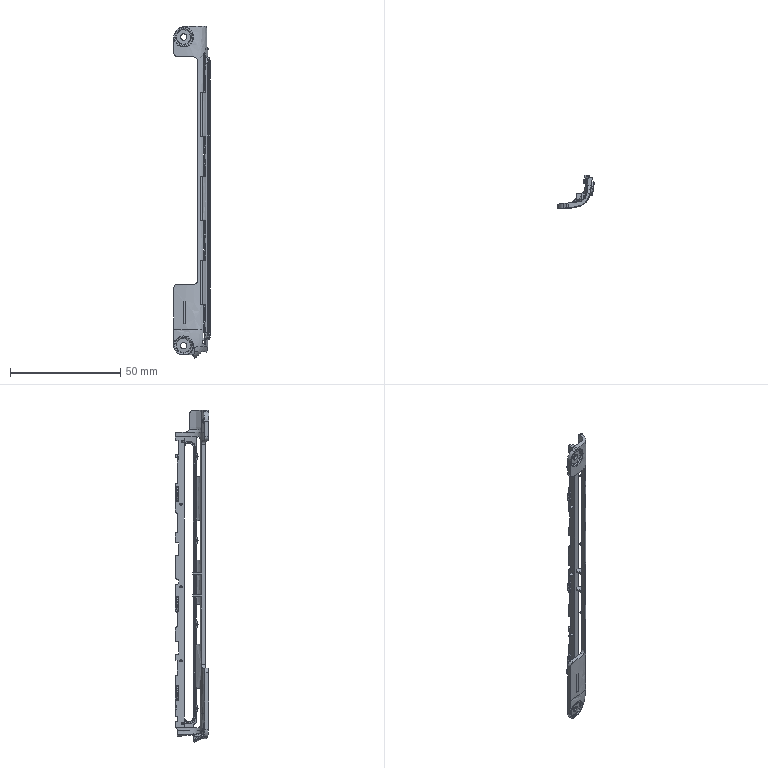Part | STEP file | SOLID | 1 solid | 430 faces | box 16.497 x 15.143 x 150.563 mm | volume 2873 mm3 | plane 166 | cylinder 129 | spline 95 | cone 20 | other 10 | torus 10 | commonest cylinder face diameters 0.6 x36 1 x25 4 x19 0.4 x11 7 x6 1.06 x4